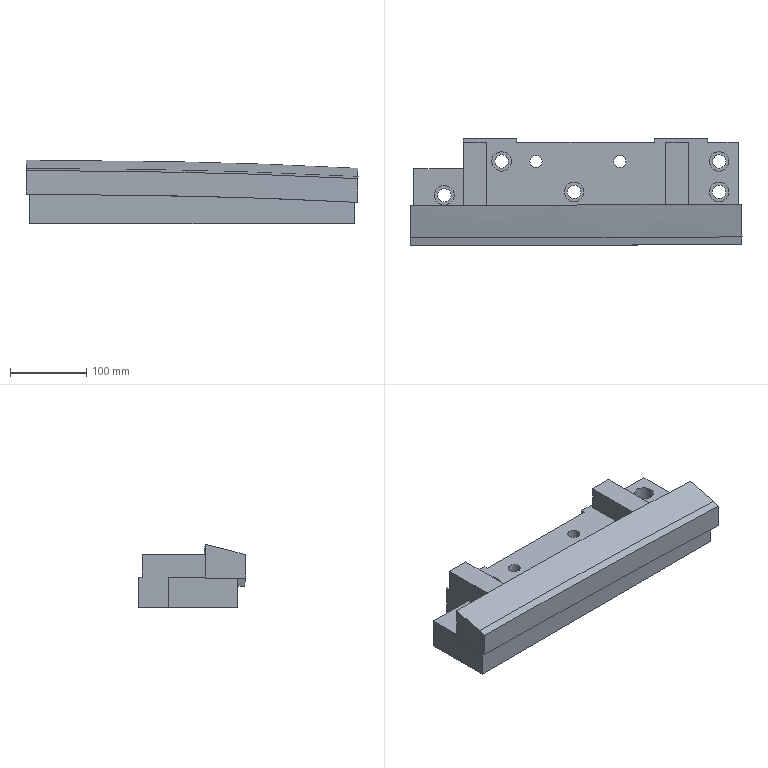Part | NX | features solid 2 | 1 solid | 47 faces | box 435 x 140.198 x 83.159 mm | volume 2897943 mm3 | plane 26 | cylinder 12 | spline 9 | commonest cylinder face diameters 17.5 x5 25.5 x4 16 x2 26 x1